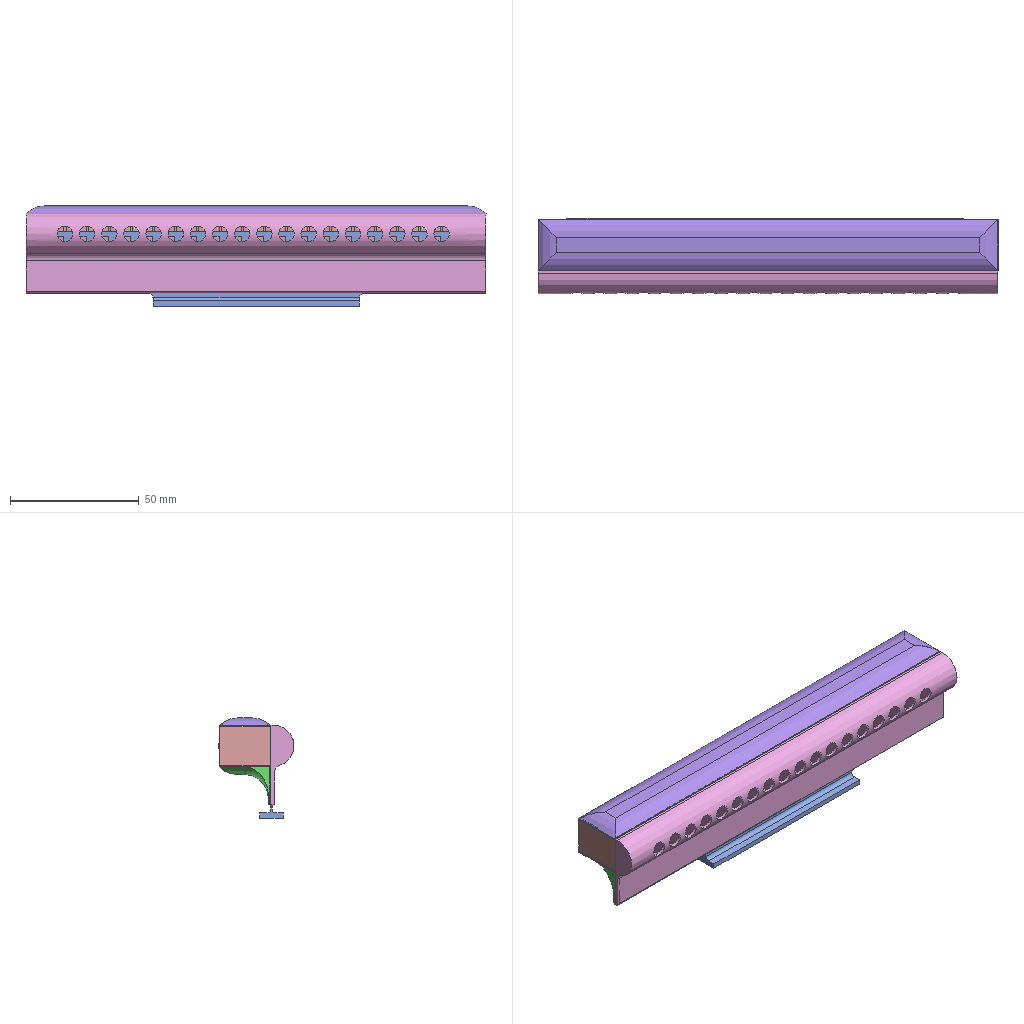Assembly | SolidWorks | 10 different items | 12 placed | box 179 x 29 x 39 mm
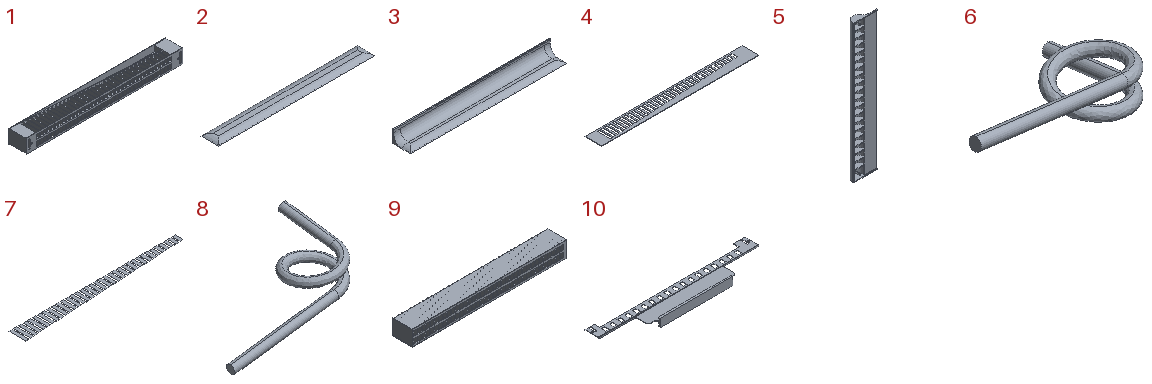Parts list (item | quantity | size | volume | features):
1 | x1 | 178.568 x 20.5 x 16 mm | 18099 mm3 | features ICE 15, Extrusion 1, MirrorPattern 1
2 | x1 | 178.57 x 20 x 3 mm | 1853 mm3 | features Extrusion 1, Fillet 1, Shell 1
3 | x1 | 178.57 x 20 x 15 mm | 6954 mm3 | features Fillet 3, ICE 2, Extrusion 1, Shell 1
4 | x2 | 178.5 x 19 x 0.5 mm | 1216 mm3 | features Extrusion 1, ICE 1
5 | x1 | 30.992 x 9 x 178.57 mm | 6725 mm3 | features ICE 5, Fillet 2, Extrusion 1, Shell 1
6 | x1 | 14.967 x 9.015 x 5.765 mm | 29.684 mm3 | features ICE 2, Helix 1, Sweep 1
7 | x2 | 153.4 x 15.412 x 0.1 mm | 115.568 mm3 | features Extrusion 1, ICE 1
8 | x1 | 14.967 x 9.015 x 5.765 mm | 29.684 mm3 | features MirrorStock 1
9 | x1 | 158.568 x 20 x 16 mm | 13194 mm3 | features ICE 3, Extrusion 1, MirrorPattern 1
10 | x1 | 176.5 x 35 x 9.08 mm | 3160 mm3 | features ICE 13, Fillet 3, Cut 1, Extrusion 1
Mates (type | each side: item.copy, entity, surface, feature):
Coincident | 1.1 face plane | 5.1 face plane Boss-Extrude2
Coincident | 1.1 face plane | 4.1 face plane Boss-Extrude1 | 2 times
DistanceDim | 4.1 face plane Cut-Extrude1 | 1.1 face plane
Coincident | 1.1 face plane | 4.2 face plane Boss-Extrude1 | 2 times
Coincident | 4.1 face plane Boss-Extrude1 | 4.2 face plane Boss-Extrude1
Coincident | 4.1 face plane Boss-Extrude1 | 7.1 face plane Boss-Extrude1
DistanceDim | 7.1 face plane Cut-Extrude1 | 4.1 face plane Cut-Extrude1
DistanceDim | 4.1 face plane Cut-Extrude1 | 7.1 face plane Cut-Extrude1
Coincident | 4.2 face plane Boss-Extrude1 | 2.1 face plane Boss-Extrude1
Coincident | 4.2 face plane Boss-Extrude1 | 2.1 edge
Coincident | 1.1 face plane | 2.1 edge
Coincident | 4.1 face plane Boss-Extrude1 | 3.1 face plane Boss-Extrude1
Coincident | 1.1 face plane | 3.1 edge | 2 times
Concentric | 1.1 face cylinder | 6.1 select_type:24
Coincident | 1.1 face plane | 5.1 face plane Boss-Extrude5
Coincident | 1.1 face plane | 10.1 face plane Boss-Extrude1